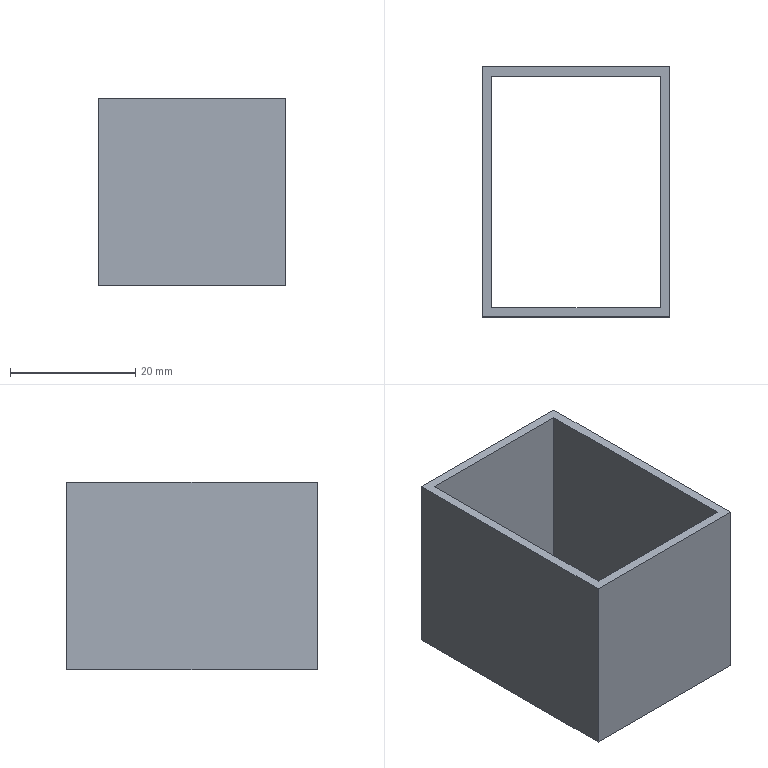Part | SolidWorks | features Extrusion 1, ICE 1 | 1 solid | 10 faces | box 30 x 40 x 30 mm | volume 6030 mm3 | plane 10
STEP:
#1=CARTESIAN_POINT('',(-37.059,39.248,0.));
#2=VERTEX_POINT('',#1);
#3=CARTESIAN_POINT('',(-37.059,-0.7524,0.));
#4=VERTEX_POINT('',#3);
#5=CARTESIAN_POINT('',(-37.059,-0.7524,0.));
#6=DIRECTION('',(0.,-1.,0.));
#7=VECTOR('',#6,1000.);
#8=LINE('',#5,#7);
#9=EDGE_CURVE('',#2,#4,#8,.T.);
#10=ORIENTED_EDGE('',*,*,#9,.T.);
#11=CARTESIAN_POINT('',(-37.059,-0.7524,30.));
#12=VERTEX_POINT('',#11);
#13=CARTESIAN_POINT('',(-37.059,-0.7524,30.));
#14=DIRECTION('',(0.,0.,-1.));
#15=VECTOR('',#14,1000.);
#16=LINE('',#13,#15);
#17=EDGE_CURVE('',#12,#4,#16,.T.);
#18=ORIENTED_EDGE('',*,*,#17,.F.);
#19=CARTESIAN_POINT('',(-37.059,39.248,30.));
#20=VERTEX_POINT('',#19);
#21=CARTESIAN_POINT('',(-37.059,-0.7524,30.));
#22=DIRECTION('',(0.,-1.,0.));
#23=VECTOR('',#22,1000.);
#24=LINE('',#21,#23);
#25=EDGE_CURVE('',#20,#12,#24,.T.);
#26=ORIENTED_EDGE('',*,*,#25,.F.);
#27=CARTESIAN_POINT('',(-37.059,39.248,30.));
#28=DIRECTION('',(0.,0.,-1.));
#29=VECTOR('',#28,1000.);
#30=LINE('',#27,#29);
#31=EDGE_CURVE('',#20,#2,#30,.T.);
#32=ORIENTED_EDGE('',*,*,#31,.T.);
#33=EDGE_LOOP('',(#10,#18,#26,#32));
#34=FACE_OUTER_BOUND('',#33,.T.);
#35=CARTESIAN_POINT('',(-37.059,-0.7524,30.));
#36=DIRECTION('',(1.,0.,0.));
#37=DIRECTION('',(0.,0.,-1.));
#38=AXIS2_PLACEMENT_3D('',#35,#36,#37);
#39=PLANE('',#38);
#40=ADVANCED_FACE('',(#34),#39,.F.);
#41=CARTESIAN_POINT('',(-7.059,-0.7524,0.));
#42=VERTEX_POINT('',#41);
#43=CARTESIAN_POINT('',(-7.059,-0.7524,0.));
#44=DIRECTION('',(1.,0.,0.));
#45=VECTOR('',#44,1000.);
#46=LINE('',#43,#45);
#47=EDGE_CURVE('',#4,#42,#46,.T.);
#48=ORIENTED_EDGE('',*,*,#47,.T.);
#49=CARTESIAN_POINT('',(-7.059,-0.7524,30.));
#50=VERTEX_POINT('',#49);
#51=CARTESIAN_POINT('',(-7.059,-0.7524,30.));
#52=DIRECTION('',(0.,0.,-1.));
#53=VECTOR('',#52,1000.);
#54=LINE('',#51,#53);
#55=EDGE_CURVE('',#50,#42,#54,.T.);
#56=ORIENTED_EDGE('',*,*,#55,.F.);
#57=CARTESIAN_POINT('',(-7.059,-0.7524,30.));
#58=DIRECTION('',(1.,0.,0.));
#59=VECTOR('',#58,1000.);
#60=LINE('',#57,#59);
#61=EDGE_CURVE('',#12,#50,#60,.T.);
#62=ORIENTED_EDGE('',*,*,#61,.F.);
#63=ORIENTED_EDGE('',*,*,#17,.T.);
#64=EDGE_LOOP('',(#48,#56,#62,#63));
#65=FACE_OUTER_BOUND('',#64,.T.);
#66=CARTESIAN_POINT('',(-7.059,-0.7524,30.));
#67=DIRECTION('',(0.,1.,0.));
#68=DIRECTION('',(0.,0.,1.));
#69=AXIS2_PLACEMENT_3D('',#66,#67,#68);
#70=PLANE('',#69);
#71=ADVANCED_FACE('',(#65),#70,.F.);
#72=CARTESIAN_POINT('',(-7.059,39.248,0.));
#73=VERTEX_POINT('',#72);
#74=CARTESIAN_POINT('',(-7.059,39.248,0.));
#75=DIRECTION('',(0.,1.,0.));
#76=VECTOR('',#75,1000.);
#77=LINE('',#74,#76);
#78=EDGE_CURVE('',#42,#73,#77,.T.);
#79=ORIENTED_EDGE('',*,*,#78,.T.);
#80=CARTESIAN_POINT('',(-7.059,39.248,30.));
#81=VERTEX_POINT('',#80);
#82=CARTESIAN_POINT('',(-7.059,39.248,30.));
#83=DIRECTION('',(0.,0.,-1.));
#84=VECTOR('',#83,1000.);
#85=LINE('',#82,#84);
#86=EDGE_CURVE('',#81,#73,#85,.T.);
#87=ORIENTED_EDGE('',*,*,#86,.F.);
#88=CARTESIAN_POINT('',(-7.059,39.248,30.));
#89=DIRECTION('',(0.,1.,0.));
#90=VECTOR('',#89,1000.);
#91=LINE('',#88,#90);
#92=EDGE_CURVE('',#50,#81,#91,.T.);
#93=ORIENTED_EDGE('',*,*,#92,.F.);
#94=ORIENTED_EDGE('',*,*,#55,.T.);
#95=EDGE_LOOP('',(#79,#87,#93,#94));
#96=FACE_OUTER_BOUND('',#95,.T.);
#97=CARTESIAN_POINT('',(-7.059,39.248,30.));
#98=DIRECTION('',(-1.,0.,0.));
#99=DIRECTION('',(0.,-1.,0.));
#100=AXIS2_PLACEMENT_3D('',#97,#98,#99);
#101=PLANE('',#100);
#102=ADVANCED_FACE('',(#96),#101,.F.);
#103=CARTESIAN_POINT('',(-37.059,39.248,0.));
#104=DIRECTION('',(-1.,0.,0.));
#105=VECTOR('',#104,1000.);
#106=LINE('',#103,#105);
#107=EDGE_CURVE('',#73,#2,#106,.T.);
#108=ORIENTED_EDGE('',*,*,#107,.T.);
#109=ORIENTED_EDGE('',*,*,#31,.F.);
#110=CARTESIAN_POINT('',(-37.059,39.248,30.));
#111=DIRECTION('',(-1.,0.,0.));
#112=VECTOR('',#111,1000.);
#113=LINE('',#110,#112);
#114=EDGE_CURVE('',#81,#20,#113,.T.);
#115=ORIENTED_EDGE('',*,*,#114,.F.);
#116=ORIENTED_EDGE('',*,*,#86,.T.);
#117=EDGE_LOOP('',(#108,#109,#115,#116));
#118=FACE_OUTER_BOUND('',#117,.T.);
#119=CARTESIAN_POINT('',(-37.059,39.248,30.));
#120=DIRECTION('',(0.,-1.,0.));
#121=DIRECTION('',(0.,0.,-1.));
#122=AXIS2_PLACEMENT_3D('',#119,#120,#121);
#123=PLANE('',#122);
#124=ADVANCED_FACE('',(#118),#123,.F.);
#125=CARTESIAN_POINT('',(-35.559,0.7476,30.));
#126=VERTEX_POINT('',#125);
#127=CARTESIAN_POINT('',(-8.559,0.7476,30.));
#128=VERTEX_POINT('',#127);
#129=CARTESIAN_POINT('',(-8.559,0.7476,30.));
#130=DIRECTION('',(1.,0.,0.));
#131=VECTOR('',#130,1000.);
#132=LINE('',#129,#131);
#133=EDGE_CURVE('',#126,#128,#132,.T.);
#134=ORIENTED_EDGE('',*,*,#133,.F.);
#135=CARTESIAN_POINT('',(-35.559,37.748,30.));
#136=VERTEX_POINT('',#135);
#137=CARTESIAN_POINT('',(-35.559,0.7476,30.));
#138=DIRECTION('',(0.,-1.,0.));
#139=VECTOR('',#138,1000.);
#140=LINE('',#137,#139);
#141=EDGE_CURVE('',#136,#126,#140,.T.);
#142=ORIENTED_EDGE('',*,*,#141,.F.);
#143=CARTESIAN_POINT('',(-8.559,37.748,30.));
#144=VERTEX_POINT('',#143);
#145=CARTESIAN_POINT('',(-35.559,37.748,30.));
#146=DIRECTION('',(-1.,0.,0.));
#147=VECTOR('',#146,1000.);
#148=LINE('',#145,#147);
#149=EDGE_CURVE('',#144,#136,#148,.T.);
#150=ORIENTED_EDGE('',*,*,#149,.F.);
#151=CARTESIAN_POINT('',(-8.559,37.748,30.));
#152=DIRECTION('',(0.,1.,0.));
#153=VECTOR('',#152,1000.);
#154=LINE('',#151,#153);
#155=EDGE_CURVE('',#128,#144,#154,.T.);
#156=ORIENTED_EDGE('',*,*,#155,.F.);
#157=EDGE_LOOP('',(#134,#142,#150,#156));
#158=FACE_BOUND('',#157,.T.);
#159=ORIENTED_EDGE('',*,*,#25,.T.);
#160=ORIENTED_EDGE('',*,*,#61,.T.);
#161=ORIENTED_EDGE('',*,*,#92,.T.);
#162=ORIENTED_EDGE('',*,*,#114,.T.);
#163=EDGE_LOOP('',(#159,#160,#161,#162));
#164=FACE_OUTER_BOUND('',#163,.T.);
#165=CARTESIAN_POINT('',(0.,0.,30.));
#166=DIRECTION('',(0.,0.,-1.));
#167=DIRECTION('',(-1.,0.,0.));
#168=AXIS2_PLACEMENT_3D('',#165,#166,#167);
#169=PLANE('',#168);
#170=ADVANCED_FACE('',(#158,#164),#169,.F.);
#171=CARTESIAN_POINT('',(-35.559,37.748,0.));
#172=VERTEX_POINT('',#171);
#173=CARTESIAN_POINT('',(-35.559,0.7476,0.));
#174=VERTEX_POINT('',#173);
#175=CARTESIAN_POINT('',(-35.559,0.7476,0.));
#176=DIRECTION('',(0.,-1.,0.));
#177=VECTOR('',#176,1000.);
#178=LINE('',#175,#177);
#179=EDGE_CURVE('',#172,#174,#178,.T.);
#180=ORIENTED_EDGE('',*,*,#179,.T.);
#181=CARTESIAN_POINT('',(-8.559,0.7476,0.));
#182=VERTEX_POINT('',#181);
#183=CARTESIAN_POINT('',(-8.559,0.7476,0.));
#184=DIRECTION('',(1.,0.,0.));
#185=VECTOR('',#184,1000.);
#186=LINE('',#183,#185);
#187=EDGE_CURVE('',#174,#182,#186,.T.);
#188=ORIENTED_EDGE('',*,*,#187,.T.);
#189=CARTESIAN_POINT('',(-8.559,37.748,0.));
#190=VERTEX_POINT('',#189);
#191=CARTESIAN_POINT('',(-8.559,37.748,0.));
#192=DIRECTION('',(0.,1.,0.));
#193=VECTOR('',#192,1000.);
#194=LINE('',#191,#193);
#195=EDGE_CURVE('',#182,#190,#194,.T.);
#196=ORIENTED_EDGE('',*,*,#195,.T.);
#197=CARTESIAN_POINT('',(-35.559,37.748,0.));
#198=DIRECTION('',(-1.,0.,0.));
#199=VECTOR('',#198,1000.);
#200=LINE('',#197,#199);
#201=EDGE_CURVE('',#190,#172,#200,.T.);
#202=ORIENTED_EDGE('',*,*,#201,.T.);
#203=EDGE_LOOP('',(#180,#188,#196,#202));
#204=FACE_BOUND('',#203,.T.);
#205=ORIENTED_EDGE('',*,*,#9,.F.);
#206=ORIENTED_EDGE('',*,*,#107,.F.);
#207=ORIENTED_EDGE('',*,*,#78,.F.);
#208=ORIENTED_EDGE('',*,*,#47,.F.);
#209=EDGE_LOOP('',(#205,#206,#207,#208));
#210=FACE_OUTER_BOUND('',#209,.T.);
#211=CARTESIAN_POINT('',(0.,0.,0.));
#212=DIRECTION('',(0.,0.,-1.));
#213=DIRECTION('',(-1.,0.,0.));
#214=AXIS2_PLACEMENT_3D('',#211,#212,#213);
#215=PLANE('',#214);
#216=ADVANCED_FACE('',(#204,#210),#215,.T.);
#217=ORIENTED_EDGE('',*,*,#141,.T.);
#218=CARTESIAN_POINT('',(-35.559,0.7476,0.));
#219=DIRECTION('',(0.,0.,1.));
#220=VECTOR('',#219,1000.);
#221=LINE('',#218,#220);
#222=EDGE_CURVE('',#174,#126,#221,.T.);
#223=ORIENTED_EDGE('',*,*,#222,.F.);
#224=ORIENTED_EDGE('',*,*,#179,.F.);
#225=CARTESIAN_POINT('',(-35.559,37.748,0.));
#226=DIRECTION('',(0.,0.,1.));
#227=VECTOR('',#226,1000.);
#228=LINE('',#225,#227);
#229=EDGE_CURVE('',#172,#136,#228,.T.);
#230=ORIENTED_EDGE('',*,*,#229,.T.);
#231=EDGE_LOOP('',(#217,#223,#224,#230));
#232=FACE_OUTER_BOUND('',#231,.T.);
#233=CARTESIAN_POINT('',(-35.559,0.7476,0.));
#234=DIRECTION('',(-1.,0.,0.));
#235=DIRECTION('',(0.,0.,1.));
#236=AXIS2_PLACEMENT_3D('',#233,#234,#235);
#237=PLANE('',#236);
#238=ADVANCED_FACE('',(#232),#237,.F.);
#239=ORIENTED_EDGE('',*,*,#149,.T.);
#240=ORIENTED_EDGE('',*,*,#229,.F.);
#241=ORIENTED_EDGE('',*,*,#201,.F.);
#242=CARTESIAN_POINT('',(-8.559,37.748,0.));
#243=DIRECTION('',(0.,0.,1.));
#244=VECTOR('',#243,1000.);
#245=LINE('',#242,#244);
#246=EDGE_CURVE('',#190,#144,#245,.T.);
#247=ORIENTED_EDGE('',*,*,#246,.T.);
#248=EDGE_LOOP('',(#239,#240,#241,#247));
#249=FACE_OUTER_BOUND('',#248,.T.);
#250=CARTESIAN_POINT('',(-35.559,37.748,0.));
#251=DIRECTION('',(0.,1.,0.));
#252=DIRECTION('',(0.,0.,1.));
#253=AXIS2_PLACEMENT_3D('',#250,#251,#252);
#254=PLANE('',#253);
#255=ADVANCED_FACE('',(#249),#254,.F.);
#256=ORIENTED_EDGE('',*,*,#155,.T.);
#257=ORIENTED_EDGE('',*,*,#246,.F.);
#258=ORIENTED_EDGE('',*,*,#195,.F.);
#259=CARTESIAN_POINT('',(-8.559,0.7476,0.));
#260=DIRECTION('',(0.,0.,1.));
#261=VECTOR('',#260,1000.);
#262=LINE('',#259,#261);
#263=EDGE_CURVE('',#182,#128,#262,.T.);
#264=ORIENTED_EDGE('',*,*,#263,.T.);
#265=EDGE_LOOP('',(#256,#257,#258,#264));
#266=FACE_OUTER_BOUND('',#265,.T.);
#267=CARTESIAN_POINT('',(-8.559,37.748,0.));
#268=DIRECTION('',(1.,0.,0.));
#269=DIRECTION('',(0.,1.,0.));
#270=AXIS2_PLACEMENT_3D('',#267,#268,#269);
#271=PLANE('',#270);
#272=ADVANCED_FACE('',(#266),#271,.F.);
#273=ORIENTED_EDGE('',*,*,#133,.T.);
#274=ORIENTED_EDGE('',*,*,#263,.F.);
#275=ORIENTED_EDGE('',*,*,#187,.F.);
#276=ORIENTED_EDGE('',*,*,#222,.T.);
#277=EDGE_LOOP('',(#273,#274,#275,#276));
#278=FACE_OUTER_BOUND('',#277,.T.);
#279=CARTESIAN_POINT('',(-8.559,0.7476,0.));
#280=DIRECTION('',(0.,-1.,0.));
#281=DIRECTION('',(1.,0.,0.));
#282=AXIS2_PLACEMENT_3D('',#279,#280,#281);
#283=PLANE('',#282);
#284=ADVANCED_FACE('',(#278),#283,.F.);
#285=CLOSED_SHELL('',(#40,#71,#102,#124,#170,#216,#238,#255,#272,#284));
#286=MANIFOLD_SOLID_BREP('',#285);
#287=CARTESIAN_POINT('',(0.,0.,0.));
#288=DIRECTION('',(0.,0.,1.));
#289=DIRECTION('',(1.,0.,0.));
#290=AXIS2_PLACEMENT_3D('',#287,#288,#289);
#291=(LENGTH_UNIT()NAMED_UNIT(*)SI_UNIT(.MILLI.,.METRE.));
#292=UNCERTAINTY_MEASURE_WITH_UNIT(LENGTH_MEASURE(0.00001),#291,'','');
#293=(NAMED_UNIT(*)PLANE_ANGLE_UNIT()SI_UNIT($,.RADIAN.));
#294=(NAMED_UNIT(*)SI_UNIT($,.STERADIAN.)SOLID_ANGLE_UNIT());
#295=(GEOMETRIC_REPRESENTATION_CONTEXT(3)GLOBAL_UNCERTAINTY_ASSIGNED_CONTEXT((#292))GLOBAL_UNIT_ASSIGNED_CONTEXT((#291,#293,#294))REPRESENTATION_CONTEXT('',''));
#296=ADVANCED_BREP_SHAPE_REPRESENTATION('',(#286,#290),#295);